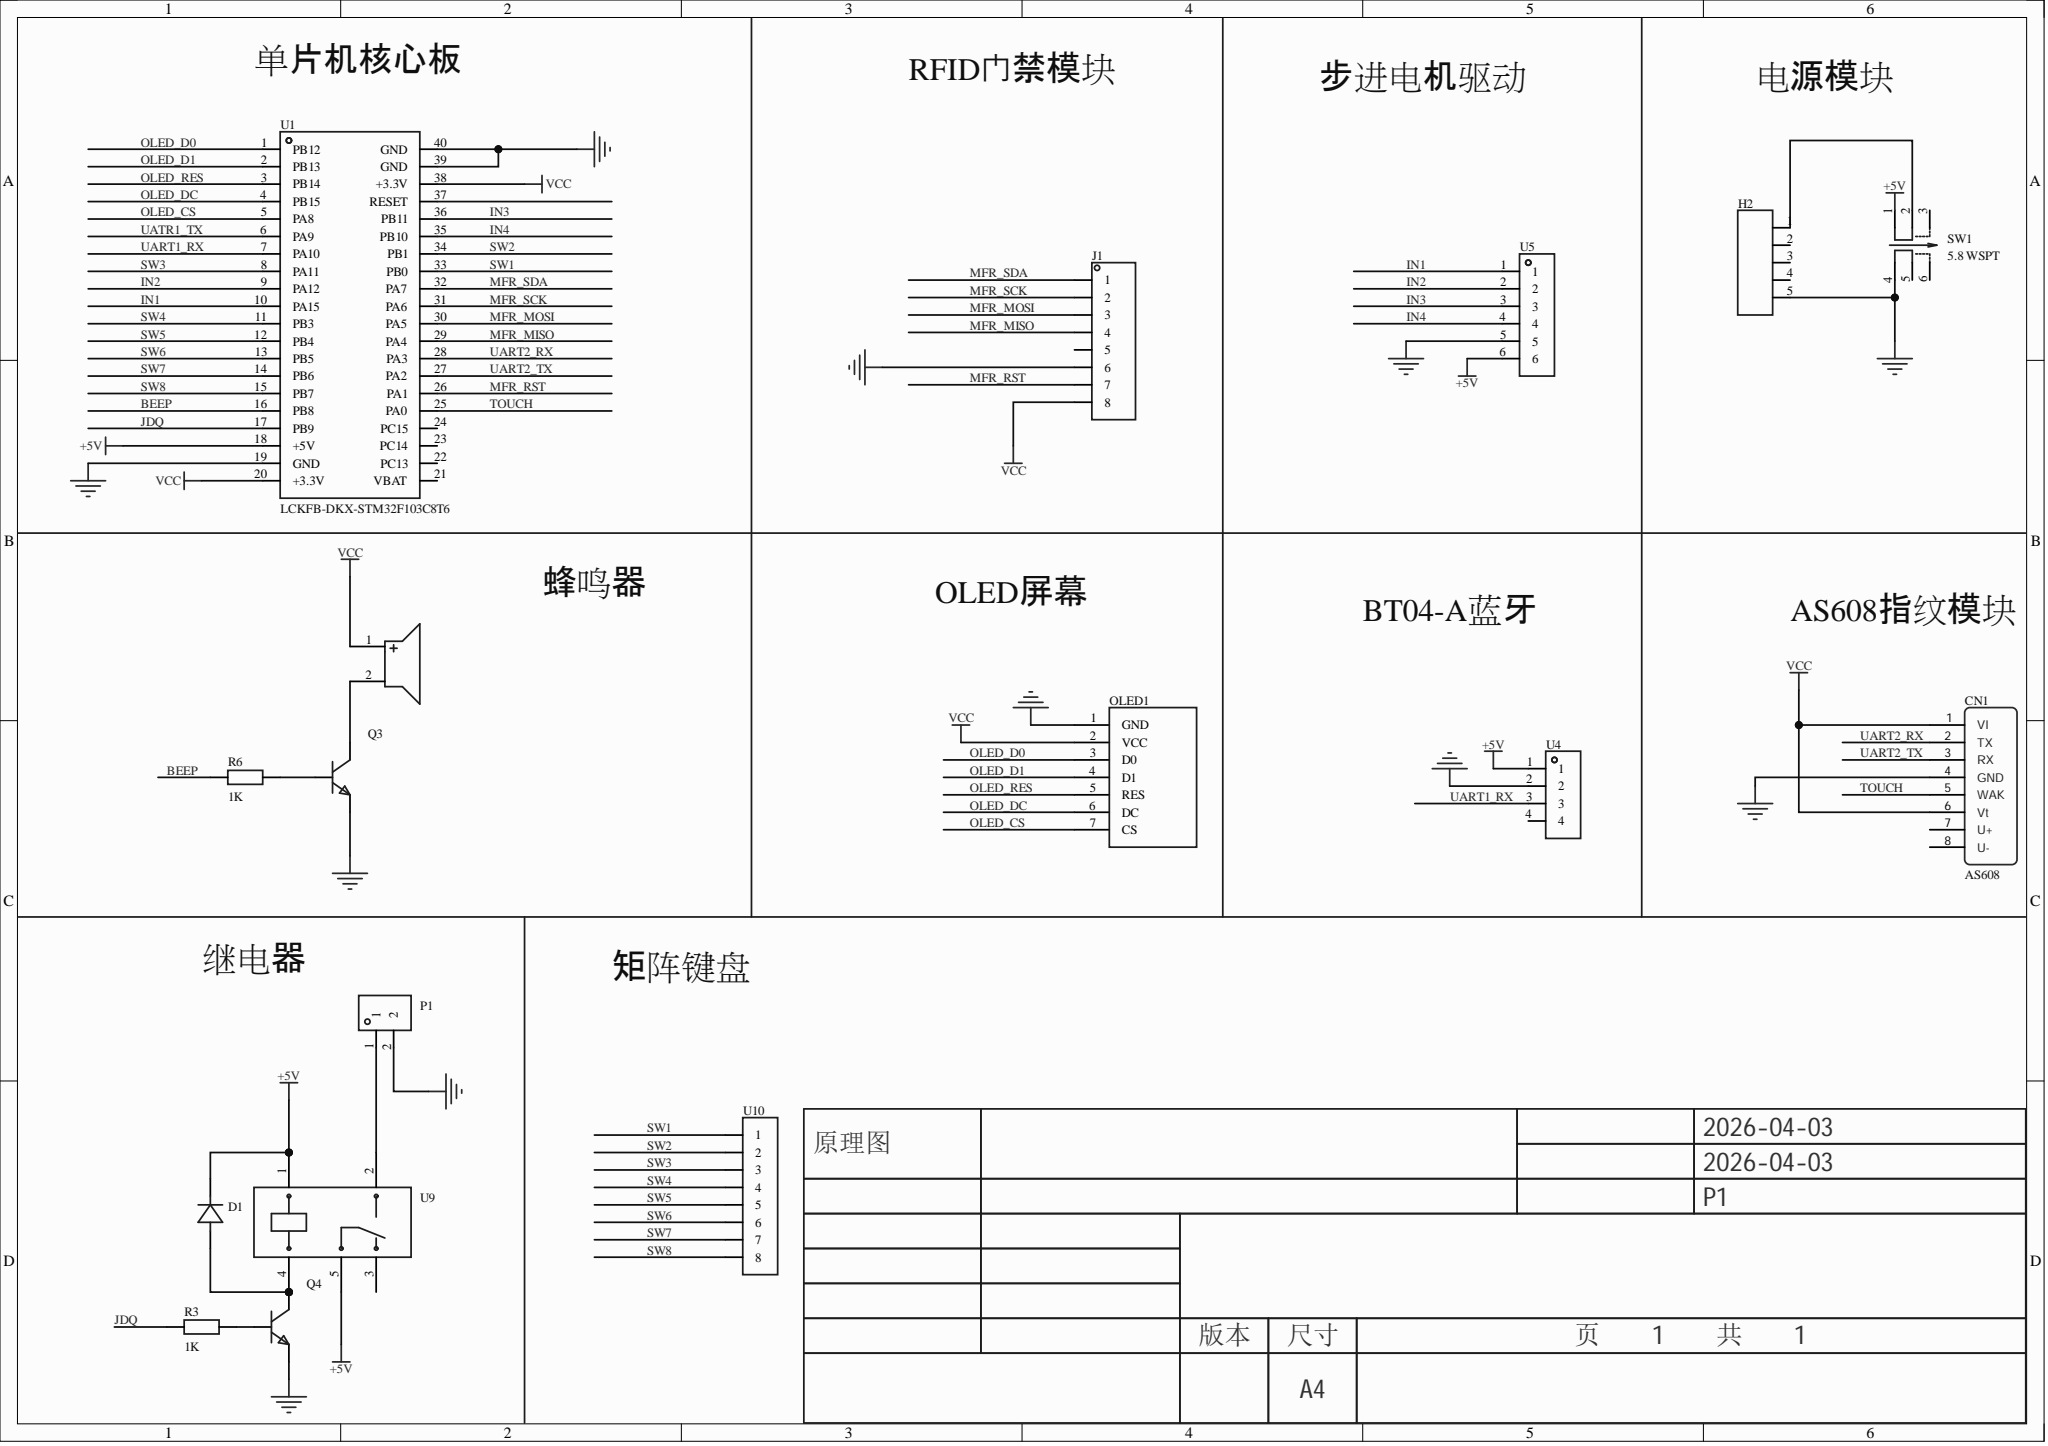Circuit board | Altium Designer | 17 parts | 37 nets
Bill of materials:
Comment,Description,Designator,Footprint,LibRef,Quantity
"2.7kHz","驱动方式:无源(外部驱动);构造类型:电磁式;频率:2.7kHz;声压(SPL):85dB;","BUZZER1","BUZ-TH_BD9.0-P4.00-D0.6-FD","QMB-09B-03","1"
"AS608","","CN1","AS608","AS608","1"
"","","D1","DO_1N4007","D_1N4007A","1"
"","","H2","HDR-TH_5P-P2.54-V-F","HDR-F_2.54_1x5P","1"
"","","J1","HDR-TH_8P-P2.54-V-M","HDR-M_2.54_1x8P","1"
"","","OLED1","0.96OLED","0.96OLED","1"
"WAFER-XH254Z-2A","插针结构:1x2P;间距:2.54mm;安装方式:直插;参考系列:XH;总PIN数:2P;排数:1;每排PIN数:2;额定电流:3A;工作温度范围:-25℃~+85℃;","P1","CONN-TH_2P-P2.50_XH-2A_3045048","WAFER-XH254Z-2A","1"
"","","Q3, Q4","S8050_TO_92","S8050_TO_NPN","2"
"1K","","R3, R6","Res_1/8W","Res_AXIAL-1/8W","2"
"5.8 WSPT","电路结构:双刀双掷;自锁/无锁:无锁;安装方式:直插;触点电流:100mA;额定电压 (AC):-;额定电压 (DC):30V;带灯:不带;作用力:1.8N;机械寿命:5千次;","SW1","SW-TH_6P-L5.8-W5.8-P2.00-LS4.5-TL_K8-5851E-L1","5.8 WSPT","1"
"LCKFB-DKX-STM32F103C8T6","","U1","CONN-TH_L53.3-W22.9_STM32F103C8T6-CARD","LCKFB-DKX-STM32F103C8T6","1"
"","","U4","HDR-TH_4P-P2.54-V-F","HDR-F_2.54_1x4P","1"
"","","U5","HDR-TH_6P-P2.54-V-F","HDR-F_2.54_1x6P","1"
"SRD-12VDC-SL-C","线圈电压:12V;触点形式:一组转换:1C(单刀双掷-转换);触点容量(电阻负载):-;最大切换电压:250V@AC;最大切换电流:15A;","U9","RELAY-TH_SRD-XXVDC-XL-C","SRD-12VDC-SL-C","1"
"","","U10","HDR-TH_8P-P2.54-V-F-1","HDR-F_2.54_1x8P","1"
Netlist (Protel format):
[
BUZZER1
BUZ-TH_BD9.0-P4.00-D0.6-FD
2.7kHz



]
[
CN1
AS608
AS608



]
[
D1
DO_1N4007




]
[
H2
HDR-TH_5P-P2.54-V-F




]
[
J1
HDR-TH_8P-P2.54-V-M




]
[
OLED1
0.96OLED




]
[
P1
CONN-TH_2P-P2.50_XH-2A_3045048
WAFER-XH254Z-2A



]
[
Q3
S8050_TO_92




]
[
Q4
S8050_TO_92




]
[
R3
Res_1/8W
1K



]
[
R6
Res_1/8W
1K



]
[
SW1
SW-TH_6P-L5.8-W5.8-P2.00-LS4.5-TL_K8-5851E-L1
5.8 WSPT



]
[
U1
CONN-TH_L53.3-W22.9_STM32F103C8T6-CARD
LCKFB-DKX-STM32F103C8T6



]
[
U4
HDR-TH_4P-P2.54-V-F




]
[
U5
HDR-TH_6P-P2.54-V-F




]
[
U9
RELAY-TH_SRD-XXVDC-XL-C
SRD-12VDC-SL-C



]
[
U10
HDR-TH_8P-P2.54-V-F-1




]
(
VCC
BUZZER1-1
CN1-1
CN1-6
J1-8
OLED1-2
U1-20
U1-38
)
(
UART2_TX
CN1-3
U1-27
)
(
UART2_RX
CN1-2
U1-28
)
(
UART1_RX
U1-7
U4-3
)
(
TOUCH
CN1-5
U1-25
)
(
SW8
U1-15
U10-8
)
(
SW7
U1-14
U10-7
)
(
SW6
U1-13
U10-6
)
(
SW5
U1-12
U10-5
)
(
SW4
U1-11
U10-4
)
(
SW3
U1-8
U10-3
)
(
SW2
U1-34
U10-2
)
(
SW1
U1-33
U10-1
)
(
OLED_RES
OLED1-5
U1-3
)
(
OLED_DC
OLED1-6
U1-4
)
(
OLED_D1
OLED1-4
U1-2
)
(
OLED_D0
OLED1-3
U1-1
)
(
OLED_CS
OLED1-7
U1-5
)
(
NetQ4_2
Q4-2
R3-2
)
(
NetQ3_2
Q3-2
R6-2
)
(
NetP1_1
P1-1
U9-2
)
(
NetH2_1
H2-1
SW1-2
)
(
NetD1_2
D1-2
Q4-3
U9-4
)
(
NetBUZZER1_2
BUZZER1-2
Q3-3
)
(
MFR_SDA
J1-1
U1-32
)
(
MFR_SCK
J1-2
U1-31
)
(
MFR_RST
J1-7
U1-26
)
(
MFR_MOSI
J1-3
U1-30
)
(
MFR_MISO
J1-4
U1-29
)
(
JDQ
R3-1
U1-17
)
(
IN4
U1-35
U5-4
)
(
IN3
U1-36
U5-3
)
(
IN2
U1-9
U5-2
)
(
IN1
U1-10
U5-1
)
(
GND
CN1-4
H2-5
J1-6
OLED1-1
P1-2
Q3-1
Q4-1
SW1-4
U1-19
U1-39
U1-40
U4-2
U5-5
)
(
BEEP
R6-1
U1-16
)
(
+5V
D1-1
SW1-1
U1-18
U4-1
U5-6
U9-1
U9-5
)